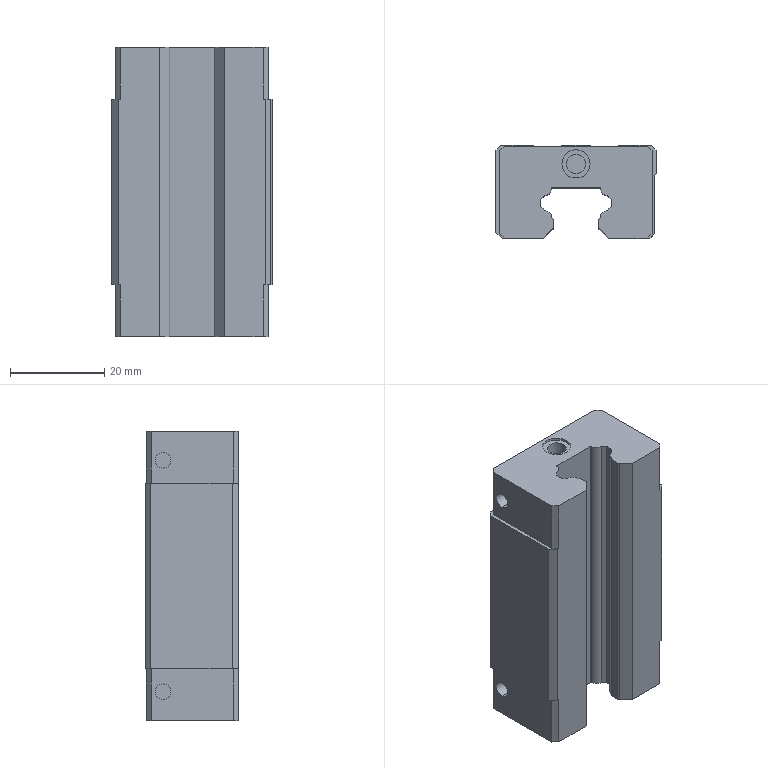Part | SolidWorks | features BaseBody 1 | 1 solid | 120 faces | box 34 x 19.7 x 61.4 mm | volume 31300 mm3 | plane 76 | cylinder 44 | commonest cylinder face diameters 4 x12 0.8 x8 3.3 x8 1 x4 3.24 x4 5.3 x4